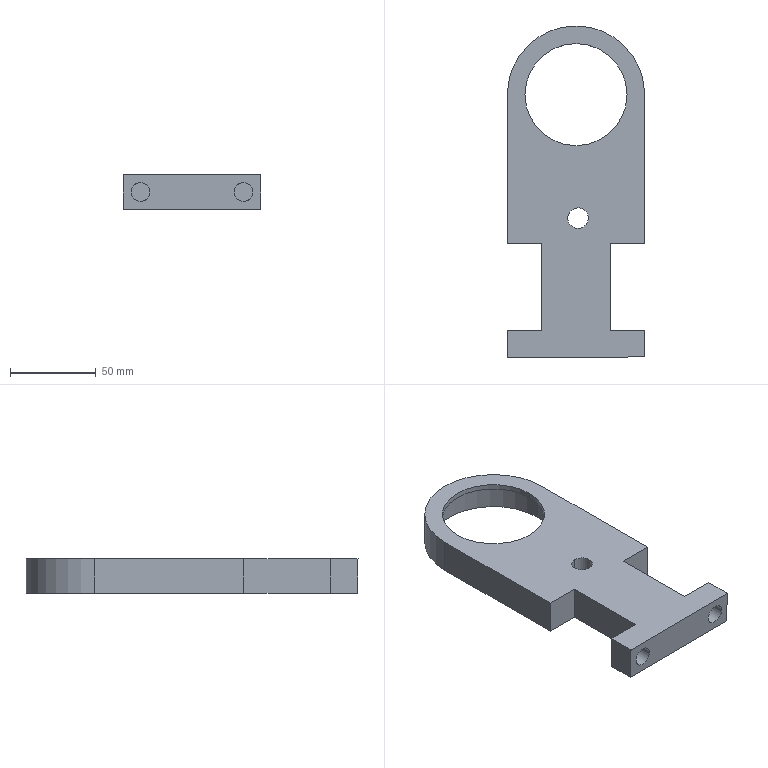Part | SolidWorks | features BaseBody 1 | 1 solid | 25 faces | box 79.997 x 193.503 x 20 mm | volume 171690 mm3 | plane 14 | cylinder 11 | commonest cylinder face diameters 11 x4 12 x2 59.5 x2 72 x2 79.997 x1
STEP:
#1=CARTESIAN_POINT('',(316.083,131.883,44.922));
#2=VERTEX_POINT('',#1);
#3=CARTESIAN_POINT('',(305.083,131.883,44.922));
#4=VERTEX_POINT('',#3);
#5=CARTESIAN_POINT('',(310.583,131.883,44.922));
#6=DIRECTION('',(0.,-1.,0.));
#7=DIRECTION('',(0.,0.,-1.));
#8=AXIS2_PLACEMENT_3D('',#5,#6,#7);
#9=CIRCLE('',#8,5.5);
#10=EDGE_CURVE('',#2,#4,#9,.T.);
#11=ORIENTED_EDGE('',*,*,#10,.F.);
#12=CARTESIAN_POINT('',(316.083,116.293,44.922));
#13=VERTEX_POINT('',#12);
#14=CARTESIAN_POINT('',(316.083,131.883,44.922));
#15=DIRECTION('',(0.,-1.,0.));
#16=VECTOR('',#15,1000.);
#17=LINE('',#14,#16);
#18=EDGE_CURVE('',#2,#13,#17,.T.);
#19=ORIENTED_EDGE('',*,*,#18,.T.);
#20=CARTESIAN_POINT('',(305.083,116.202,44.922));
#21=VERTEX_POINT('',#20);
#22=CARTESIAN_POINT('',(305.083,116.202,44.922));
#23=CARTESIAN_POINT('',(305.083,115.892,55.922));
#24=CARTESIAN_POINT('',(316.083,115.983,55.922));
#25=CARTESIAN_POINT('',(316.083,116.293,44.922));
#26=(BOUNDED_CURVE()B_SPLINE_CURVE(3,(#22,#23,#24,#25),.UNSPECIFIED.,.F.,.F.)B_SPLINE_CURVE_WITH_KNOTS((4,4),(4.999,8.14),.UNSPECIFIED.)CURVE()GEOMETRIC_REPRESENTATION_ITEM()RATIONAL_B_SPLINE_CURVE((1.,0.3333,0.3333,1.))REPRESENTATION_ITEM(''));
#27=EDGE_CURVE('',#21,#13,#26,.T.);
#28=ORIENTED_EDGE('',*,*,#27,.F.);
#29=CARTESIAN_POINT('',(305.083,131.883,44.922));
#30=DIRECTION('',(0.,-1.,0.));
#31=VECTOR('',#30,1000.);
#32=LINE('',#29,#31);
#33=EDGE_CURVE('',#4,#21,#32,.T.);
#34=ORIENTED_EDGE('',*,*,#33,.F.);
#35=EDGE_LOOP('',(#11,#19,#28,#34));
#36=FACE_OUTER_BOUND('',#35,.T.);
#37=CARTESIAN_POINT('',(310.583,131.883,44.922));
#38=DIRECTION('',(0.,-1.,0.));
#39=DIRECTION('',(-1.,0.,0.));
#40=AXIS2_PLACEMENT_3D('',#37,#38,#39);
#41=CYLINDRICAL_SURFACE('',#40,5.5);
#42=ADVANCED_FACE('',(#36),#41,.F.);
#43=CARTESIAN_POINT('',(365.083,131.883,44.922));
#44=VERTEX_POINT('',#43);
#45=CARTESIAN_POINT('',(376.083,131.883,44.922));
#46=VERTEX_POINT('',#45);
#47=CARTESIAN_POINT('',(370.583,131.883,44.922));
#48=DIRECTION('',(0.000000015,-1.,0.));
#49=DIRECTION('',(-1.,-0.000000015,0.));
#50=AXIS2_PLACEMENT_3D('',#47,#48,#49);
#51=CIRCLE('',#50,5.5);
#52=EDGE_CURVE('',#44,#46,#51,.T.);
#53=ORIENTED_EDGE('',*,*,#52,.F.);
#54=CARTESIAN_POINT('',(365.083,116.698,44.922));
#55=VERTEX_POINT('',#54);
#56=CARTESIAN_POINT('',(365.083,131.883,44.922));
#57=DIRECTION('',(0.000000015,-1.,0.));
#58=VECTOR('',#57,1000.);
#59=LINE('',#56,#58);
#60=EDGE_CURVE('',#44,#55,#59,.T.);
#61=ORIENTED_EDGE('',*,*,#60,.T.);
#62=CARTESIAN_POINT('',(376.083,116.789,44.922));
#63=VERTEX_POINT('',#62);
#64=CARTESIAN_POINT('',(376.083,116.789,44.922));
#65=CARTESIAN_POINT('',(376.083,117.099,33.922));
#66=CARTESIAN_POINT('',(365.083,117.008,33.922));
#67=CARTESIAN_POINT('',(365.083,116.698,44.922));
#68=(BOUNDED_CURVE()B_SPLINE_CURVE(3,(#64,#65,#66,#67),.UNSPECIFIED.,.F.,.F.)B_SPLINE_CURVE_WITH_KNOTS((4,4),(1.857,4.999),.UNSPECIFIED.)CURVE()GEOMETRIC_REPRESENTATION_ITEM()RATIONAL_B_SPLINE_CURVE((1.,0.3333,0.3333,1.))REPRESENTATION_ITEM(''));
#69=EDGE_CURVE('',#63,#55,#68,.T.);
#70=ORIENTED_EDGE('',*,*,#69,.F.);
#71=CARTESIAN_POINT('',(376.083,131.883,44.922));
#72=DIRECTION('',(0.000000015,-1.,0.));
#73=VECTOR('',#72,1000.);
#74=LINE('',#71,#73);
#75=EDGE_CURVE('',#46,#63,#74,.T.);
#76=ORIENTED_EDGE('',*,*,#75,.F.);
#77=EDGE_LOOP('',(#53,#61,#70,#76));
#78=FACE_OUTER_BOUND('',#77,.T.);
#79=CARTESIAN_POINT('',(370.583,131.883,44.922));
#80=DIRECTION('',(0.000000015,-1.,0.));
#81=DIRECTION('',(1.,0.000000015,0.));
#82=AXIS2_PLACEMENT_3D('',#79,#80,#81);
#83=CYLINDRICAL_SURFACE('',#82,5.5);
#84=ADVANCED_FACE('',(#78),#83,.F.);
#85=CARTESIAN_POINT('',(341.89,191.405,54.922));
#86=VERTEX_POINT('',#85);
#87=CARTESIAN_POINT('',(341.637,203.402,54.922));
#88=VERTEX_POINT('',#87);
#89=CARTESIAN_POINT('',(341.89,191.405,54.922));
#90=CARTESIAN_POINT('',(353.887,191.657,54.922));
#91=CARTESIAN_POINT('',(353.635,203.655,54.922));
#92=CARTESIAN_POINT('',(341.637,203.402,54.922));
#93=(BOUNDED_CURVE()B_SPLINE_CURVE(3,(#89,#90,#91,#92),.UNSPECIFIED.,.F.,.F.)B_SPLINE_CURVE_WITH_KNOTS((4,4),(4.73,7.871),.UNSPECIFIED.)CURVE()GEOMETRIC_REPRESENTATION_ITEM()RATIONAL_B_SPLINE_CURVE((1.,0.3333,0.3333,1.))REPRESENTATION_ITEM(''));
#94=EDGE_CURVE('',#86,#88,#93,.T.);
#95=ORIENTED_EDGE('',*,*,#94,.T.);
#96=CARTESIAN_POINT('',(341.64,203.402,34.922));
#97=VERTEX_POINT('',#96);
#98=CARTESIAN_POINT('',(341.643,203.402,19.726));
#99=DIRECTION('',(0.0001435,0.000000521,-1.));
#100=VECTOR('',#99,1000.);
#101=LINE('',#98,#100);
#102=EDGE_CURVE('',#88,#97,#101,.T.);
#103=ORIENTED_EDGE('',*,*,#102,.T.);
#104=CARTESIAN_POINT('',(341.893,191.405,34.922));
#105=VERTEX_POINT('',#104);
#106=CARTESIAN_POINT('',(341.893,191.405,34.922));
#107=CARTESIAN_POINT('',(353.89,191.657,34.922));
#108=CARTESIAN_POINT('',(353.638,203.655,34.922));
#109=CARTESIAN_POINT('',(341.64,203.402,34.922));
#110=(BOUNDED_CURVE()B_SPLINE_CURVE(3,(#106,#107,#108,#109),.UNSPECIFIED.,.F.,.F.)B_SPLINE_CURVE_WITH_KNOTS((4,4),(4.73,7.871),.UNSPECIFIED.)CURVE()GEOMETRIC_REPRESENTATION_ITEM()RATIONAL_B_SPLINE_CURVE((1.,0.3333,0.3333,1.))REPRESENTATION_ITEM(''));
#111=EDGE_CURVE('',#105,#97,#110,.T.);
#112=ORIENTED_EDGE('',*,*,#111,.F.);
#113=CARTESIAN_POINT('',(341.895,191.405,19.726));
#114=DIRECTION('',(0.0001435,0.000000521,-1.));
#115=VECTOR('',#114,1000.);
#116=LINE('',#113,#115);
#117=EDGE_CURVE('',#86,#105,#116,.T.);
#118=ORIENTED_EDGE('',*,*,#117,.F.);
#119=EDGE_LOOP('',(#95,#103,#112,#118));
#120=FACE_OUTER_BOUND('',#119,.T.);
#121=CARTESIAN_POINT('',(341.769,197.404,19.726));
#122=DIRECTION('',(0.0001435,0.000000521,-1.));
#123=DIRECTION('',(0.02104,-0.9998,0.000002497));
#124=AXIS2_PLACEMENT_3D('',#121,#122,#123);
#125=CYLINDRICAL_SURFACE('',#124,6.);
#126=ADVANCED_FACE('',(#120),#125,.F.);
#127=CARTESIAN_POINT('',(310.833,269.388,51.922));
#128=VERTEX_POINT('',#127);
#129=CARTESIAN_POINT('',(370.333,269.388,51.922));
#130=VERTEX_POINT('',#129);
#131=CARTESIAN_POINT('',(340.583,269.388,51.922));
#132=DIRECTION('',(0.,0.,1.));
#133=DIRECTION('',(-1.,-0.000000008,0.));
#134=AXIS2_PLACEMENT_3D('',#131,#132,#133);
#135=CIRCLE('',#134,29.75);
#136=EDGE_CURVE('',#128,#130,#135,.T.);
#137=ORIENTED_EDGE('',*,*,#136,.F.);
#138=CARTESIAN_POINT('',(310.833,269.388,54.922));
#139=VERTEX_POINT('',#138);
#140=CARTESIAN_POINT('',(310.833,269.388,51.922));
#141=DIRECTION('',(0.,0.,1.));
#142=VECTOR('',#141,1000.);
#143=LINE('',#140,#142);
#144=EDGE_CURVE('',#128,#139,#143,.T.);
#145=ORIENTED_EDGE('',*,*,#144,.T.);
#146=CARTESIAN_POINT('',(370.333,269.388,54.922));
#147=VERTEX_POINT('',#146);
#148=CARTESIAN_POINT('',(340.583,269.388,54.922));
#149=DIRECTION('',(0.,0.,-1.));
#150=DIRECTION('',(-1.,-0.000000008,0.));
#151=AXIS2_PLACEMENT_3D('',#148,#149,#150);
#152=CIRCLE('',#151,29.75);
#153=EDGE_CURVE('',#147,#139,#152,.T.);
#154=ORIENTED_EDGE('',*,*,#153,.F.);
#155=CARTESIAN_POINT('',(370.333,269.388,51.922));
#156=DIRECTION('',(0.,0.,1.));
#157=VECTOR('',#156,1000.);
#158=LINE('',#155,#157);
#159=EDGE_CURVE('',#130,#147,#158,.T.);
#160=ORIENTED_EDGE('',*,*,#159,.F.);
#161=EDGE_LOOP('',(#137,#145,#154,#160));
#162=FACE_OUTER_BOUND('',#161,.T.);
#163=CARTESIAN_POINT('',(340.583,269.388,51.922));
#164=DIRECTION('',(0.,0.,1.));
#165=DIRECTION('',(1.,0.000000008,0.));
#166=AXIS2_PLACEMENT_3D('',#163,#164,#165);
#167=CYLINDRICAL_SURFACE('',#166,29.75);
#168=ADVANCED_FACE('',(#162),#167,.F.);
#169=CARTESIAN_POINT('',(304.583,269.388,34.922));
#170=VERTEX_POINT('',#169);
#171=CARTESIAN_POINT('',(376.583,269.388,34.922));
#172=VERTEX_POINT('',#171);
#173=CARTESIAN_POINT('',(340.583,269.388,34.922));
#174=DIRECTION('',(0.,0.,1.));
#175=DIRECTION('',(-1.,-0.000000007,0.));
#176=AXIS2_PLACEMENT_3D('',#173,#174,#175);
#177=CIRCLE('',#176,36.);
#178=EDGE_CURVE('',#170,#172,#177,.T.);
#179=ORIENTED_EDGE('',*,*,#178,.F.);
#180=CARTESIAN_POINT('',(304.583,269.388,51.922));
#181=VERTEX_POINT('',#180);
#182=CARTESIAN_POINT('',(304.583,269.388,-93.078));
#183=DIRECTION('',(0.,0.,1.));
#184=VECTOR('',#183,1000.);
#185=LINE('',#182,#184);
#186=EDGE_CURVE('',#170,#181,#185,.T.);
#187=ORIENTED_EDGE('',*,*,#186,.T.);
#188=CARTESIAN_POINT('',(376.583,269.388,51.922));
#189=VERTEX_POINT('',#188);
#190=CARTESIAN_POINT('',(340.583,269.388,51.922));
#191=DIRECTION('',(0.,0.,-1.));
#192=DIRECTION('',(-1.,-0.000000007,0.));
#193=AXIS2_PLACEMENT_3D('',#190,#191,#192);
#194=CIRCLE('',#193,36.);
#195=EDGE_CURVE('',#189,#181,#194,.T.);
#196=ORIENTED_EDGE('',*,*,#195,.F.);
#197=CARTESIAN_POINT('',(376.583,269.388,-93.078));
#198=DIRECTION('',(0.,0.,1.));
#199=VECTOR('',#198,1000.);
#200=LINE('',#197,#199);
#201=EDGE_CURVE('',#172,#189,#200,.T.);
#202=ORIENTED_EDGE('',*,*,#201,.F.);
#203=EDGE_LOOP('',(#179,#187,#196,#202));
#204=FACE_OUTER_BOUND('',#203,.T.);
#205=CARTESIAN_POINT('',(340.583,269.388,-93.078));
#206=DIRECTION('',(0.,0.,1.));
#207=DIRECTION('',(1.,0.000000007,0.));
#208=AXIS2_PLACEMENT_3D('',#205,#206,#207);
#209=CYLINDRICAL_SURFACE('',#208,36.);
#210=ADVANCED_FACE('',(#204),#209,.F.);
#211=ORIENTED_EDGE('',*,*,#186,.F.);
#212=CARTESIAN_POINT('',(340.583,269.388,34.922));
#213=DIRECTION('',(0.,0.,1.));
#214=DIRECTION('',(-1.,-0.000000007,0.));
#215=AXIS2_PLACEMENT_3D('',#212,#213,#214);
#216=CIRCLE('',#215,36.);
#217=EDGE_CURVE('',#172,#170,#216,.T.);
#218=ORIENTED_EDGE('',*,*,#217,.F.);
#219=ORIENTED_EDGE('',*,*,#201,.T.);
#220=CARTESIAN_POINT('',(340.583,269.388,51.922));
#221=DIRECTION('',(0.,0.,-1.));
#222=DIRECTION('',(-1.,-0.000000007,0.));
#223=AXIS2_PLACEMENT_3D('',#220,#221,#222);
#224=CIRCLE('',#223,36.);
#225=EDGE_CURVE('',#181,#189,#224,.T.);
#226=ORIENTED_EDGE('',*,*,#225,.F.);
#227=EDGE_LOOP('',(#211,#218,#219,#226));
#228=FACE_OUTER_BOUND('',#227,.T.);
#229=CARTESIAN_POINT('',(340.583,269.388,-93.078));
#230=DIRECTION('',(0.,0.,1.));
#231=DIRECTION('',(1.,0.000000007,0.));
#232=AXIS2_PLACEMENT_3D('',#229,#230,#231);
#233=CYLINDRICAL_SURFACE('',#232,36.);
#234=ADVANCED_FACE('',(#228),#233,.F.);
#235=CARTESIAN_POINT('',(340.583,269.388,51.922));
#236=DIRECTION('',(0.,0.,1.));
#237=DIRECTION('',(-1.,-0.000000008,0.));
#238=AXIS2_PLACEMENT_3D('',#235,#236,#237);
#239=CIRCLE('',#238,29.75);
#240=EDGE_CURVE('',#130,#128,#239,.T.);
#241=ORIENTED_EDGE('',*,*,#240,.T.);
#242=ORIENTED_EDGE('',*,*,#136,.T.);
#243=EDGE_LOOP('',(#241,#242));
#244=FACE_BOUND('',#243,.T.);
#245=ORIENTED_EDGE('',*,*,#195,.T.);
#246=ORIENTED_EDGE('',*,*,#225,.T.);
#247=EDGE_LOOP('',(#245,#246));
#248=FACE_OUTER_BOUND('',#247,.T.);
#249=CARTESIAN_POINT('',(340.583,269.388,51.922));
#250=DIRECTION('',(0.,0.,1.));
#251=DIRECTION('',(0.,-1.,0.));
#252=AXIS2_PLACEMENT_3D('',#249,#250,#251);
#253=PLANE('',#252);
#254=ADVANCED_FACE('',(#244,#248),#253,.F.);
#255=ORIENTED_EDGE('',*,*,#144,.F.);
#256=ORIENTED_EDGE('',*,*,#240,.F.);
#257=ORIENTED_EDGE('',*,*,#159,.T.);
#258=CARTESIAN_POINT('',(340.583,269.388,54.922));
#259=DIRECTION('',(0.,0.,-1.));
#260=DIRECTION('',(-1.,-0.000000008,0.));
#261=AXIS2_PLACEMENT_3D('',#258,#259,#260);
#262=CIRCLE('',#261,29.75);
#263=EDGE_CURVE('',#139,#147,#262,.T.);
#264=ORIENTED_EDGE('',*,*,#263,.F.);
#265=EDGE_LOOP('',(#255,#256,#257,#264));
#266=FACE_OUTER_BOUND('',#265,.T.);
#267=CARTESIAN_POINT('',(340.583,269.388,51.922));
#268=DIRECTION('',(0.,0.,1.));
#269=DIRECTION('',(1.,0.000000008,0.));
#270=AXIS2_PLACEMENT_3D('',#267,#268,#269);
#271=CYLINDRICAL_SURFACE('',#270,29.75);
#272=ADVANCED_FACE('',(#266),#271,.F.);
#273=CARTESIAN_POINT('',(360.583,182.446,54.922));
#274=VERTEX_POINT('',#273);
#275=CARTESIAN_POINT('',(360.583,182.446,34.922));
#276=VERTEX_POINT('',#275);
#277=CARTESIAN_POINT('',(360.583,182.446,54.922));
#278=DIRECTION('',(0.,0.,-1.));
#279=VECTOR('',#278,1000.);
#280=LINE('',#277,#279);
#281=EDGE_CURVE('',#274,#276,#280,.T.);
#282=ORIENTED_EDGE('',*,*,#281,.F.);
#283=CARTESIAN_POINT('',(360.583,131.883,54.922));
#284=VERTEX_POINT('',#283);
#285=CARTESIAN_POINT('',(360.583,131.883,54.922));
#286=DIRECTION('',(-0.000000015,1.,0.));
#287=VECTOR('',#286,1000.);
#288=LINE('',#285,#287);
#289=EDGE_CURVE('',#284,#274,#288,.T.);
#290=ORIENTED_EDGE('',*,*,#289,.F.);
#291=CARTESIAN_POINT('',(360.583,131.883,34.922));
#292=VERTEX_POINT('',#291);
#293=CARTESIAN_POINT('',(360.583,131.883,54.922));
#294=DIRECTION('',(0.,0.,-1.));
#295=VECTOR('',#294,1000.);
#296=LINE('',#293,#295);
#297=EDGE_CURVE('',#284,#292,#296,.T.);
#298=ORIENTED_EDGE('',*,*,#297,.T.);
#299=CARTESIAN_POINT('',(360.583,182.446,34.922));
#300=DIRECTION('',(0.000000015,-1.,0.));
#301=VECTOR('',#300,1000.);
#302=LINE('',#299,#301);
#303=EDGE_CURVE('',#276,#292,#302,.T.);
#304=ORIENTED_EDGE('',*,*,#303,.F.);
#305=EDGE_LOOP('',(#282,#290,#298,#304));
#306=FACE_OUTER_BOUND('',#305,.T.);
#307=CARTESIAN_POINT('',(360.583,151.164,14.922));
#308=DIRECTION('',(-1.,-0.000000015,0.));
#309=DIRECTION('',(-0.000000015,1.,0.));
#310=AXIS2_PLACEMENT_3D('',#307,#308,#309);
#311=PLANE('',#310);
#312=ADVANCED_FACE('',(#306),#311,.F.);
#313=CARTESIAN_POINT('',(380.582,182.446,54.922));
#314=VERTEX_POINT('',#313);
#315=CARTESIAN_POINT('',(380.582,182.446,34.922));
#316=VERTEX_POINT('',#315);
#317=CARTESIAN_POINT('',(380.582,182.446,54.922));
#318=DIRECTION('',(0.,0.,-1.));
#319=VECTOR('',#318,1000.);
#320=LINE('',#317,#319);
#321=EDGE_CURVE('',#314,#316,#320,.T.);
#322=ORIENTED_EDGE('',*,*,#321,.F.);
#323=CARTESIAN_POINT('',(360.583,182.446,54.922));
#324=DIRECTION('',(1.,0.000000015,0.));
#325=VECTOR('',#324,1000.);
#326=LINE('',#323,#325);
#327=EDGE_CURVE('',#274,#314,#326,.T.);
#328=ORIENTED_EDGE('',*,*,#327,.F.);
#329=ORIENTED_EDGE('',*,*,#281,.T.);
#330=CARTESIAN_POINT('',(380.582,182.446,34.922));
#331=DIRECTION('',(-1.,-0.000000015,0.));
#332=VECTOR('',#331,1000.);
#333=LINE('',#330,#332);
#334=EDGE_CURVE('',#316,#276,#333,.T.);
#335=ORIENTED_EDGE('',*,*,#334,.F.);
#336=EDGE_LOOP('',(#322,#328,#329,#335));
#337=FACE_OUTER_BOUND('',#336,.T.);
#338=CARTESIAN_POINT('',(380.583,182.446,14.922));
#339=DIRECTION('',(-0.000000015,1.,0.));
#340=DIRECTION('',(0.,0.,1.));
#341=AXIS2_PLACEMENT_3D('',#338,#339,#340);
#342=PLANE('',#341);
#343=ADVANCED_FACE('',(#337),#342,.F.);
#344=CARTESIAN_POINT('',(380.582,269.388,34.922));
#345=VERTEX_POINT('',#344);
#346=CARTESIAN_POINT('',(380.582,269.388,34.922));
#347=DIRECTION('',(0.000000008,-1.,0.));
#348=VECTOR('',#347,1000.);
#349=LINE('',#346,#348);
#350=EDGE_CURVE('',#345,#316,#349,.T.);
#351=ORIENTED_EDGE('',*,*,#350,.F.);
#352=CARTESIAN_POINT('',(380.582,269.388,54.922));
#353=VERTEX_POINT('',#352);
#354=CARTESIAN_POINT('',(380.582,269.388,54.922));
#355=DIRECTION('',(0.,0.,-1.));
#356=VECTOR('',#355,1000.);
#357=LINE('',#354,#356);
#358=EDGE_CURVE('',#353,#345,#357,.T.);
#359=ORIENTED_EDGE('',*,*,#358,.F.);
#360=CARTESIAN_POINT('',(380.582,182.446,54.922));
#361=DIRECTION('',(-0.000000008,1.,0.));
#362=VECTOR('',#361,1000.);
#363=LINE('',#360,#362);
#364=EDGE_CURVE('',#314,#353,#363,.T.);
#365=ORIENTED_EDGE('',*,*,#364,.F.);
#366=ORIENTED_EDGE('',*,*,#321,.T.);
#367=EDGE_LOOP('',(#351,#359,#365,#366));
#368=FACE_OUTER_BOUND('',#367,.T.);
#369=CARTESIAN_POINT('',(380.582,208.23,62.809));
#370=DIRECTION('',(1.,0.000000008,0.));
#371=DIRECTION('',(0.,0.,-1.));
#372=AXIS2_PLACEMENT_3D('',#369,#370,#371);
#373=PLANE('',#372);
#374=ADVANCED_FACE('',(#368),#373,.T.);
#375=CARTESIAN_POINT('',(300.585,269.388,54.922));
#376=VERTEX_POINT('',#375);
#377=CARTESIAN_POINT('',(340.583,269.388,54.922));
#378=DIRECTION('',(0.,0.,1.));
#379=DIRECTION('',(1.,0.,0.));
#380=AXIS2_PLACEMENT_3D('',#377,#378,#379);
#381=CIRCLE('',#380,39.999);
#382=EDGE_CURVE('',#353,#376,#381,.T.);
#383=ORIENTED_EDGE('',*,*,#382,.F.);
#384=ORIENTED_EDGE('',*,*,#358,.T.);
#385=CARTESIAN_POINT('',(300.585,269.388,34.922));
#386=VERTEX_POINT('',#385);
#387=CARTESIAN_POINT('',(340.583,269.388,34.922));
#388=DIRECTION('',(0.,0.,-1.));
#389=DIRECTION('',(-1.,0.,0.));
#390=AXIS2_PLACEMENT_3D('',#387,#388,#389);
#391=CIRCLE('',#390,39.999);
#392=EDGE_CURVE('',#386,#345,#391,.T.);
#393=ORIENTED_EDGE('',*,*,#392,.F.);
#394=CARTESIAN_POINT('',(300.585,269.388,34.922));
#395=DIRECTION('',(0.,0.,1.));
#396=VECTOR('',#395,1000.);
#397=LINE('',#394,#396);
#398=EDGE_CURVE('',#386,#376,#397,.T.);
#399=ORIENTED_EDGE('',*,*,#398,.T.);
#400=EDGE_LOOP('',(#383,#384,#393,#399));
#401=FACE_OUTER_BOUND('',#400,.T.);
#402=CARTESIAN_POINT('',(340.583,269.388,62.817));
#403=DIRECTION('',(0.,0.,-1.));
#404=DIRECTION('',(-1.,-0.000000007,0.));
#405=AXIS2_PLACEMENT_3D('',#402,#403,#404);
#406=CYLINDRICAL_SURFACE('',#405,39.999);
#407=ADVANCED_FACE('',(#401),#406,.T.);
#408=CARTESIAN_POINT('',(300.585,182.446,54.922));
#409=VERTEX_POINT('',#408);
#410=CARTESIAN_POINT('',(300.585,269.388,54.922));
#411=DIRECTION('',(0.000000008,-1.,0.));
#412=VECTOR('',#411,1000.);
#413=LINE('',#410,#412);
#414=EDGE_CURVE('',#376,#409,#413,.T.);
#415=ORIENTED_EDGE('',*,*,#414,.F.);
#416=ORIENTED_EDGE('',*,*,#398,.F.);
#417=CARTESIAN_POINT('',(300.585,182.446,34.922));
#418=VERTEX_POINT('',#417);
#419=CARTESIAN_POINT('',(300.585,182.446,34.922));
#420=DIRECTION('',(-0.000000008,1.,0.));
#421=VECTOR('',#420,1000.);
#422=LINE('',#419,#421);
#423=EDGE_CURVE('',#418,#386,#422,.T.);
#424=ORIENTED_EDGE('',*,*,#423,.F.);
#425=CARTESIAN_POINT('',(300.585,182.446,34.922));
#426=DIRECTION('',(0.,0.,1.));
#427=VECTOR('',#426,1000.);
#428=LINE('',#425,#427);
#429=EDGE_CURVE('',#418,#409,#428,.T.);
#430=ORIENTED_EDGE('',*,*,#429,.T.);
#431=EDGE_LOOP('',(#415,#416,#424,#430));
#432=FACE_OUTER_BOUND('',#431,.T.);
#433=CARTESIAN_POINT('',(300.585,208.23,62.817));
#434=DIRECTION('',(-1.,-0.000000008,0.));
#435=DIRECTION('',(-0.000000008,1.,0.));
#436=AXIS2_PLACEMENT_3D('',#433,#434,#435);
#437=PLANE('',#436);
#438=ADVANCED_FACE('',(#432),#437,.T.);
#439=CARTESIAN_POINT('',(320.583,182.446,34.922));
#440=VERTEX_POINT('',#439);
#441=CARTESIAN_POINT('',(320.583,182.446,54.922));
#442=VERTEX_POINT('',#441);
#443=CARTESIAN_POINT('',(320.583,182.446,34.922));
#444=DIRECTION('',(0.,0.,1.));
#445=VECTOR('',#444,1000.);
#446=LINE('',#443,#445);
#447=EDGE_CURVE('',#440,#442,#446,.T.);
#448=ORIENTED_EDGE('',*,*,#447,.T.);
#449=CARTESIAN_POINT('',(300.585,182.446,54.922));
#450=DIRECTION('',(1.,0.,0.));
#451=VECTOR('',#450,1000.);
#452=LINE('',#449,#451);
#453=EDGE_CURVE('',#409,#442,#452,.T.);
#454=ORIENTED_EDGE('',*,*,#453,.F.);
#455=ORIENTED_EDGE('',*,*,#429,.F.);
#456=CARTESIAN_POINT('',(320.583,182.446,34.922));
#457=DIRECTION('',(-1.,0.,0.));
#458=VECTOR('',#457,1000.);
#459=LINE('',#456,#458);
#460=EDGE_CURVE('',#440,#418,#459,.T.);
#461=ORIENTED_EDGE('',*,*,#460,.F.);
#462=EDGE_LOOP('',(#448,#454,#455,#461));
#463=FACE_OUTER_BOUND('',#462,.T.);
#464=CARTESIAN_POINT('',(300.583,182.446,14.922));
#465=DIRECTION('',(0.,1.,0.));
#466=DIRECTION('',(1.,0.,0.));
#467=AXIS2_PLACEMENT_3D('',#464,#465,#466);
#468=PLANE('',#467);
#469=ADVANCED_FACE('',(#463),#468,.F.);
#470=CARTESIAN_POINT('',(320.583,131.883,34.922));
#471=VERTEX_POINT('',#470);
#472=CARTESIAN_POINT('',(320.583,131.883,54.922));
#473=VERTEX_POINT('',#472);
#474=CARTESIAN_POINT('',(320.583,131.883,34.922));
#475=DIRECTION('',(0.,0.,1.));
#476=VECTOR('',#475,1000.);
#477=LINE('',#474,#476);
#478=EDGE_CURVE('',#471,#473,#477,.T.);
#479=ORIENTED_EDGE('',*,*,#478,.T.);
#480=CARTESIAN_POINT('',(320.583,182.446,54.922));
#481=DIRECTION('',(0.,-1.,0.));
#482=VECTOR('',#481,1000.);
#483=LINE('',#480,#482);
#484=EDGE_CURVE('',#442,#473,#483,.T.);
#485=ORIENTED_EDGE('',*,*,#484,.F.);
#486=ORIENTED_EDGE('',*,*,#447,.F.);
#487=CARTESIAN_POINT('',(320.583,131.883,34.922));
#488=DIRECTION('',(0.,1.,0.));
#489=VECTOR('',#488,1000.);
#490=LINE('',#487,#489);
#491=EDGE_CURVE('',#471,#440,#490,.T.);
#492=ORIENTED_EDGE('',*,*,#491,.F.);
#493=EDGE_LOOP('',(#479,#485,#486,#492));
#494=FACE_OUTER_BOUND('',#493,.T.);
#495=CARTESIAN_POINT('',(320.583,151.164,14.922));
#496=DIRECTION('',(1.,0.,0.));
#497=DIRECTION('',(0.,1.,0.));
#498=AXIS2_PLACEMENT_3D('',#495,#496,#497);
#499=PLANE('',#498);
#500=ADVANCED_FACE('',(#494),#499,.F.);
#501=CARTESIAN_POINT('',(300.585,116.446,34.922));
#502=VERTEX_POINT('',#501);
#503=CARTESIAN_POINT('',(300.585,131.883,34.922));
#504=VERTEX_POINT('',#503);
#505=CARTESIAN_POINT('',(300.585,116.446,34.922));
#506=DIRECTION('',(-0.000000008,1.,0.));
#507=VECTOR('',#506,1000.);
#508=LINE('',#505,#507);
#509=EDGE_CURVE('',#502,#504,#508,.T.);
#510=ORIENTED_EDGE('',*,*,#509,.F.);
#511=CARTESIAN_POINT('',(300.585,115.883,54.922));
#512=VERTEX_POINT('',#511);
#513=CARTESIAN_POINT('',(300.585,116.446,34.922));
#514=DIRECTION('',(0.,-0.02812,0.9996));
#515=VECTOR('',#514,1000.);
#516=LINE('',#513,#515);
#517=EDGE_CURVE('',#502,#512,#516,.T.);
#518=ORIENTED_EDGE('',*,*,#517,.T.);
#519=CARTESIAN_POINT('',(300.585,131.883,54.922));
#520=VERTEX_POINT('',#519);
#521=CARTESIAN_POINT('',(300.585,131.883,54.922));
#522=DIRECTION('',(0.000000008,-1.,0.));
#523=VECTOR('',#522,1000.);
#524=LINE('',#521,#523);
#525=EDGE_CURVE('',#520,#512,#524,.T.);
#526=ORIENTED_EDGE('',*,*,#525,.F.);
#527=CARTESIAN_POINT('',(300.585,131.883,54.922));
#528=DIRECTION('',(0.,0.,-1.));
#529=VECTOR('',#528,1000.);
#530=LINE('',#527,#529);
#531=EDGE_CURVE('',#520,#504,#530,.T.);
#532=ORIENTED_EDGE('',*,*,#531,.T.);
#533=EDGE_LOOP('',(#510,#518,#526,#532));
#534=FACE_OUTER_BOUND('',#533,.T.);
#535=CARTESIAN_POINT('',(300.585,208.23,62.817));
#536=DIRECTION('',(-1.,-0.000000008,0.));
#537=DIRECTION('',(-0.000000008,1.,0.));
#538=AXIS2_PLACEMENT_3D('',#535,#536,#537);
#539=PLANE('',#538);
#540=ADVANCED_FACE('',(#534),#539,.T.);
#541=ORIENTED_EDGE('',*,*,#102,.F.);
#542=CARTESIAN_POINT('',(341.637,203.402,54.922));
#543=CARTESIAN_POINT('',(329.64,203.15,54.922));
#544=CARTESIAN_POINT('',(329.893,191.152,54.922));
#545=CARTESIAN_POINT('',(341.89,191.405,54.922));
#546=(BOUNDED_CURVE()B_SPLINE_CURVE(3,(#542,#543,#544,#545),.UNSPECIFIED.,.F.,.F.)B_SPLINE_CURVE_WITH_KNOTS((4,4),(1.588,4.73),.UNSPECIFIED.)CURVE()GEOMETRIC_REPRESENTATION_ITEM()RATIONAL_B_SPLINE_CURVE((1.,0.3333,0.3333,1.))REPRESENTATION_ITEM(''));
#547=EDGE_CURVE('',#88,#86,#546,.T.);
#548=ORIENTED_EDGE('',*,*,#547,.T.);
#549=ORIENTED_EDGE('',*,*,#117,.T.);
#550=CARTESIAN_POINT('',(341.64,203.402,34.922));
#551=CARTESIAN_POINT('',(329.643,203.15,34.922));
#552=CARTESIAN_POINT('',(329.895,191.152,34.922));
#553=CARTESIAN_POINT('',(341.893,191.405,34.922));
#554=(BOUNDED_CURVE()B_SPLINE_CURVE(3,(#550,#551,#552,#553),.UNSPECIFIED.,.F.,.F.)B_SPLINE_CURVE_WITH_KNOTS((4,4),(1.588,4.73),.UNSPECIFIED.)CURVE()GEOMETRIC_REPRESENTATION_ITEM()RATIONAL_B_SPLINE_CURVE((1.,0.3333,0.3333,1.))REPRESENTATION_ITEM(''));
#555=EDGE_CURVE('',#97,#105,#554,.T.);
#556=ORIENTED_EDGE('',*,*,#555,.F.);
#557=EDGE_LOOP('',(#541,#548,#549,#556));
#558=FACE_OUTER_BOUND('',#557,.T.);
#559=CARTESIAN_POINT('',(341.769,197.404,19.726));
#560=DIRECTION('',(0.0001435,0.000000521,-1.));
#561=DIRECTION('',(0.02104,-0.9998,0.000002497));
#562=AXIS2_PLACEMENT_3D('',#559,#560,#561);
#563=CYLINDRICAL_SURFACE('',#562,6.);
#564=ADVANCED_FACE('',(#558),#563,.F.);
#565=ORIENTED_EDGE('',*,*,#153,.T.);
#566=ORIENTED_EDGE('',*,*,#263,.T.);
#567=EDGE_LOOP('',(#565,#566));
#568=FACE_BOUND('',#567,.T.);
#569=ORIENTED_EDGE('',*,*,#94,.F.);
#570=ORIENTED_EDGE('',*,*,#547,.F.);
#571=EDGE_LOOP('',(#569,#570));
#572=FACE_BOUND('',#571,.T.);
#573=ORIENTED_EDGE('',*,*,#289,.T.);
#574=ORIENTED_EDGE('',*,*,#327,.T.);
#575=ORIENTED_EDGE('',*,*,#364,.T.);
#576=ORIENTED_EDGE('',*,*,#382,.T.);
#577=ORIENTED_EDGE('',*,*,#414,.T.);
#578=ORIENTED_EDGE('',*,*,#453,.T.);
#579=ORIENTED_EDGE('',*,*,#484,.T.);
#580=CARTESIAN_POINT('',(320.583,131.883,54.922));
#581=DIRECTION('',(-1.,0.,0.));
#582=VECTOR('',#581,1000.);
#583=LINE('',#580,#582);
#584=EDGE_CURVE('',#473,#520,#583,.T.);
#585=ORIENTED_EDGE('',*,*,#584,.T.);
#586=ORIENTED_EDGE('',*,*,#525,.T.);
#587=CARTESIAN_POINT('',(380.582,116.545,54.922));
#588=VERTEX_POINT('',#587);
#589=CARTESIAN_POINT('',(300.585,115.883,54.922));
#590=DIRECTION('',(1.,0.008278,0.));
#591=VECTOR('',#590,1000.);
#592=LINE('',#589,#591);
#593=EDGE_CURVE('',#512,#588,#592,.T.);
#594=ORIENTED_EDGE('',*,*,#593,.T.);
#595=CARTESIAN_POINT('',(380.582,131.883,54.922));
#596=VERTEX_POINT('',#595);
#597=CARTESIAN_POINT('',(380.582,116.545,54.922));
#598=DIRECTION('',(-0.000000008,1.,0.));
#599=VECTOR('',#598,1000.);
#600=LINE('',#597,#599);
#601=EDGE_CURVE('',#588,#596,#600,.T.);
#602=ORIENTED_EDGE('',*,*,#601,.T.);
#603=CARTESIAN_POINT('',(380.582,131.883,54.922));
#604=DIRECTION('',(-1.,-0.000000015,0.));
#605=VECTOR('',#604,1000.);
#606=LINE('',#603,#605);
#607=EDGE_CURVE('',#596,#284,#606,.T.);
#608=ORIENTED_EDGE('',*,*,#607,.T.);
#609=EDGE_LOOP('',(#573,#574,#575,#576,#577,#578,#579,#585,#586,#594,#602,#608));
#610=FACE_OUTER_BOUND('',#609,.T.);
#611=CARTESIAN_POINT('',(330.292,234.89,54.922));
#612=DIRECTION('',(0.,0.,1.));
#613=DIRECTION('',(1.,0.,0.));
#614=AXIS2_PLACEMENT_3D('',#611,#612,#613);
#615=PLANE('',#614);
#616=ADVANCED_FACE('',(#568,#572,#610),#615,.T.);
#617=ORIENTED_EDGE('',*,*,#601,.F.);
#618=CARTESIAN_POINT('',(380.582,117.108,34.922));
#619=VERTEX_POINT('',#618);
#620=CARTESIAN_POINT('',(380.582,116.545,54.922));
#621=DIRECTION('',(0.,0.02812,-0.9996));
#622=VECTOR('',#621,1000.);
#623=LINE('',#620,#622);
#624=EDGE_CURVE('',#588,#619,#623,.T.);
#625=ORIENTED_EDGE('',*,*,#624,.T.);
#626=CARTESIAN_POINT('',(380.582,131.883,34.922));
#627=VERTEX_POINT('',#626);
#628=CARTESIAN_POINT('',(380.582,131.883,34.922));
#629=DIRECTION('',(0.000000008,-1.,0.));
#630=VECTOR('',#629,1000.);
#631=LINE('',#628,#630);
#632=EDGE_CURVE('',#627,#619,#631,.T.);
#633=ORIENTED_EDGE('',*,*,#632,.F.);
#634=CARTESIAN_POINT('',(380.582,131.883,34.922));
#635=DIRECTION('',(0.,0.,1.));
#636=VECTOR('',#635,1000.);
#637=LINE('',#634,#636);
#638=EDGE_CURVE('',#627,#596,#637,.T.);
#639=ORIENTED_EDGE('',*,*,#638,.T.);
#640=EDGE_LOOP('',(#617,#625,#633,#639));
#641=FACE_OUTER_BOUND('',#640,.T.);
#642=CARTESIAN_POINT('',(380.582,208.23,62.809));
#643=DIRECTION('',(1.,0.000000008,0.));
#644=DIRECTION('',(0.,0.,-1.));
#645=AXIS2_PLACEMENT_3D('',#642,#643,#644);
#646=PLANE('',#645);
#647=ADVANCED_FACE('',(#641),#646,.T.);
#648=ORIENTED_EDGE('',*,*,#60,.F.);
#649=CARTESIAN_POINT('',(370.583,131.883,44.922));
#650=DIRECTION('',(0.000000015,-1.,0.));
#651=DIRECTION('',(-1.,-0.000000015,0.));
#652=AXIS2_PLACEMENT_3D('',#649,#650,#651);
#653=CIRCLE('',#652,5.5);
#654=EDGE_CURVE('',#46,#44,#653,.T.);
#655=ORIENTED_EDGE('',*,*,#654,.F.);
#656=ORIENTED_EDGE('',*,*,#75,.T.);
#657=CARTESIAN_POINT('',(365.083,116.698,44.922));
#658=CARTESIAN_POINT('',(365.083,116.389,55.922));
#659=CARTESIAN_POINT('',(376.083,116.48,55.922));
#660=CARTESIAN_POINT('',(376.083,116.789,44.922));
#661=(BOUNDED_CURVE()B_SPLINE_CURVE(3,(#657,#658,#659,#660),.UNSPECIFIED.,.F.,.F.)B_SPLINE_CURVE_WITH_KNOTS((4,4),(4.999,8.14),.UNSPECIFIED.)CURVE()GEOMETRIC_REPRESENTATION_ITEM()RATIONAL_B_SPLINE_CURVE((1.,0.3333,0.3333,1.))REPRESENTATION_ITEM(''));
#662=EDGE_CURVE('',#55,#63,#661,.T.);
#663=ORIENTED_EDGE('',*,*,#662,.F.);
#664=EDGE_LOOP('',(#648,#655,#656,#663));
#665=FACE_OUTER_BOUND('',#664,.T.);
#666=CARTESIAN_POINT('',(370.583,131.883,44.922));
#667=DIRECTION('',(0.000000015,-1.,0.));
#668=DIRECTION('',(1.,0.000000015,0.));
#669=AXIS2_PLACEMENT_3D('',#666,#667,#668);
#670=CYLINDRICAL_SURFACE('',#669,5.5);
#671=ADVANCED_FACE('',(#665),#670,.F.);
#672=ORIENTED_EDGE('',*,*,#654,.T.);
#673=ORIENTED_EDGE('',*,*,#52,.T.);
#674=EDGE_LOOP('',(#672,#673));
#675=FACE_BOUND('',#674,.T.);
#676=ORIENTED_EDGE('',*,*,#297,.F.);
#677=ORIENTED_EDGE('',*,*,#607,.F.);
#678=ORIENTED_EDGE('',*,*,#638,.F.);
#679=CARTESIAN_POINT('',(360.583,131.883,34.922));
#680=DIRECTION('',(1.,0.000000015,0.));
#681=VECTOR('',#680,1000.);
#682=LINE('',#679,#681);
#683=EDGE_CURVE('',#292,#627,#682,.T.);
#684=ORIENTED_EDGE('',*,*,#683,.F.);
#685=EDGE_LOOP('',(#676,#677,#678,#684));
#686=FACE_OUTER_BOUND('',#685,.T.);
#687=CARTESIAN_POINT('',(380.583,131.883,14.922));
#688=DIRECTION('',(0.000000015,-1.,0.));
#689=DIRECTION('',(0.,0.,-1.));
#690=AXIS2_PLACEMENT_3D('',#687,#688,#689);
#691=PLANE('',#690);
#692=ADVANCED_FACE('',(#675,#686),#691,.F.);
#693=ORIENTED_EDGE('',*,*,#217,.T.);
#694=ORIENTED_EDGE('',*,*,#178,.T.);
#695=EDGE_LOOP('',(#693,#694));
#696=FACE_BOUND('',#695,.T.);
#697=ORIENTED_EDGE('',*,*,#111,.T.);
#698=ORIENTED_EDGE('',*,*,#555,.T.);
#699=EDGE_LOOP('',(#697,#698));
#700=FACE_BOUND('',#699,.T.);
#701=ORIENTED_EDGE('',*,*,#632,.T.);
#702=CARTESIAN_POINT('',(380.582,117.108,34.922));
#703=DIRECTION('',(-1.,-0.008278,0.));
#704=VECTOR('',#703,1000.);
#705=LINE('',#702,#704);
#706=EDGE_CURVE('',#619,#502,#705,.T.);
#707=ORIENTED_EDGE('',*,*,#706,.T.);
#708=ORIENTED_EDGE('',*,*,#509,.T.);
#709=CARTESIAN_POINT('',(300.585,131.883,34.922));
#710=DIRECTION('',(1.,0.,0.));
#711=VECTOR('',#710,1000.);
#712=LINE('',#709,#711);
#713=EDGE_CURVE('',#504,#471,#712,.T.);
#714=ORIENTED_EDGE('',*,*,#713,.T.);
#715=ORIENTED_EDGE('',*,*,#491,.T.);
#716=ORIENTED_EDGE('',*,*,#460,.T.);
#717=ORIENTED_EDGE('',*,*,#423,.T.);
#718=ORIENTED_EDGE('',*,*,#392,.T.);
#719=ORIENTED_EDGE('',*,*,#350,.T.);
#720=ORIENTED_EDGE('',*,*,#334,.T.);
#721=ORIENTED_EDGE('',*,*,#303,.T.);
#722=ORIENTED_EDGE('',*,*,#683,.T.);
#723=EDGE_LOOP('',(#701,#707,#708,#714,#715,#716,#717,#718,#719,#720,#721,#722));
#724=FACE_OUTER_BOUND('',#723,.T.);
#725=CARTESIAN_POINT('',(330.292,234.89,34.922));
#726=DIRECTION('',(0.,0.,1.));
#727=DIRECTION('',(1.,0.,0.));
#728=AXIS2_PLACEMENT_3D('',#725,#726,#727);
#729=PLANE('',#728);
#730=ADVANCED_FACE('',(#696,#700,#724),#729,.F.);
#731=CARTESIAN_POINT('',(310.583,131.883,44.922));
#732=DIRECTION('',(0.,-1.,0.));
#733=DIRECTION('',(0.,0.,-1.));
#734=AXIS2_PLACEMENT_3D('',#731,#732,#733);
#735=CIRCLE('',#734,5.5);
#736=EDGE_CURVE('',#4,#2,#735,.T.);
#737=ORIENTED_EDGE('',*,*,#736,.T.);
#738=ORIENTED_EDGE('',*,*,#10,.T.);
#739=EDGE_LOOP('',(#737,#738));
#740=FACE_BOUND('',#739,.T.);
#741=ORIENTED_EDGE('',*,*,#531,.F.);
#742=ORIENTED_EDGE('',*,*,#584,.F.);
#743=ORIENTED_EDGE('',*,*,#478,.F.);
#744=ORIENTED_EDGE('',*,*,#713,.F.);
#745=EDGE_LOOP('',(#741,#742,#743,#744));
#746=FACE_OUTER_BOUND('',#745,.T.);
#747=CARTESIAN_POINT('',(300.583,131.883,14.922));
#748=DIRECTION('',(0.,-1.,0.));
#749=DIRECTION('',(0.,0.,-1.));
#750=AXIS2_PLACEMENT_3D('',#747,#748,#749);
#751=PLANE('',#750);
#752=ADVANCED_FACE('',(#740,#746),#751,.F.);
#753=ORIENTED_EDGE('',*,*,#27,.T.);
#754=CARTESIAN_POINT('',(316.083,116.293,44.922));
#755=CARTESIAN_POINT('',(316.083,116.602,33.922));
#756=CARTESIAN_POINT('',(305.083,116.511,33.922));
#757=CARTESIAN_POINT('',(305.083,116.202,44.922));
#758=(BOUNDED_CURVE()B_SPLINE_CURVE(3,(#754,#755,#756,#757),.UNSPECIFIED.,.F.,.F.)B_SPLINE_CURVE_WITH_KNOTS((4,4),(1.857,4.999),.UNSPECIFIED.)CURVE()GEOMETRIC_REPRESENTATION_ITEM()RATIONAL_B_SPLINE_CURVE((1.,0.3333,0.3333,1.))REPRESENTATION_ITEM(''));
#759=EDGE_CURVE('',#13,#21,#758,.T.);
#760=ORIENTED_EDGE('',*,*,#759,.T.);
#761=EDGE_LOOP('',(#753,#760));
#762=FACE_BOUND('',#761,.T.);
#763=ORIENTED_EDGE('',*,*,#69,.T.);
#764=ORIENTED_EDGE('',*,*,#662,.T.);
#765=EDGE_LOOP('',(#763,#764));
#766=FACE_BOUND('',#765,.T.);
#767=ORIENTED_EDGE('',*,*,#706,.F.);
#768=ORIENTED_EDGE('',*,*,#624,.F.);
#769=ORIENTED_EDGE('',*,*,#593,.F.);
#770=ORIENTED_EDGE('',*,*,#517,.F.);
#771=EDGE_LOOP('',(#767,#768,#769,#770));
#772=FACE_OUTER_BOUND('',#771,.T.);
#773=CARTESIAN_POINT('',(623.797,120.56,-16.201));
#774=DIRECTION('',(-0.008275,0.9996,0.02812));
#775=DIRECTION('',(0.9593,0.,0.2823));
#776=AXIS2_PLACEMENT_3D('',#773,#774,#775);
#777=PLANE('',#776);
#778=ADVANCED_FACE('',(#762,#766,#772),#777,.F.);
#779=ORIENTED_EDGE('',*,*,#18,.F.);
#780=ORIENTED_EDGE('',*,*,#736,.F.);
#781=ORIENTED_EDGE('',*,*,#33,.T.);
#782=ORIENTED_EDGE('',*,*,#759,.F.);
#783=EDGE_LOOP('',(#779,#780,#781,#782));
#784=FACE_OUTER_BOUND('',#783,.T.);
#785=CARTESIAN_POINT('',(310.583,131.883,44.922));
#786=DIRECTION('',(0.,-1.,0.));
#787=DIRECTION('',(-1.,0.,0.));
#788=AXIS2_PLACEMENT_3D('',#785,#786,#787);
#789=CYLINDRICAL_SURFACE('',#788,5.5);
#790=ADVANCED_FACE('',(#784),#789,.F.);
#791=CLOSED_SHELL('',(#42,#84,#126,#168,#210,#234,#254,#272,#312,#343,#374,#407,#438,#469,#500,#540,#564,#616,#647,#671,#692,#730,#752,#778,#790));
#792=MANIFOLD_SOLID_BREP('',#791);
#793=CARTESIAN_POINT('',(0.,0.,0.));
#794=DIRECTION('',(0.,0.,1.));
#795=DIRECTION('',(1.,0.,0.));
#796=AXIS2_PLACEMENT_3D('',#793,#794,#795);
#797=(LENGTH_UNIT()NAMED_UNIT(*)SI_UNIT(.MILLI.,.METRE.));
#798=UNCERTAINTY_MEASURE_WITH_UNIT(LENGTH_MEASURE(0.00001),#797,'','');
#799=(NAMED_UNIT(*)PLANE_ANGLE_UNIT()SI_UNIT($,.RADIAN.));
#800=(NAMED_UNIT(*)SI_UNIT($,.STERADIAN.)SOLID_ANGLE_UNIT());
#801=(GEOMETRIC_REPRESENTATION_CONTEXT(3)GLOBAL_UNCERTAINTY_ASSIGNED_CONTEXT((#798))GLOBAL_UNIT_ASSIGNED_CONTEXT((#797,#799,#800))REPRESENTATION_CONTEXT('',''));
#802=ADVANCED_BREP_SHAPE_REPRESENTATION('',(#792,#796),#801);